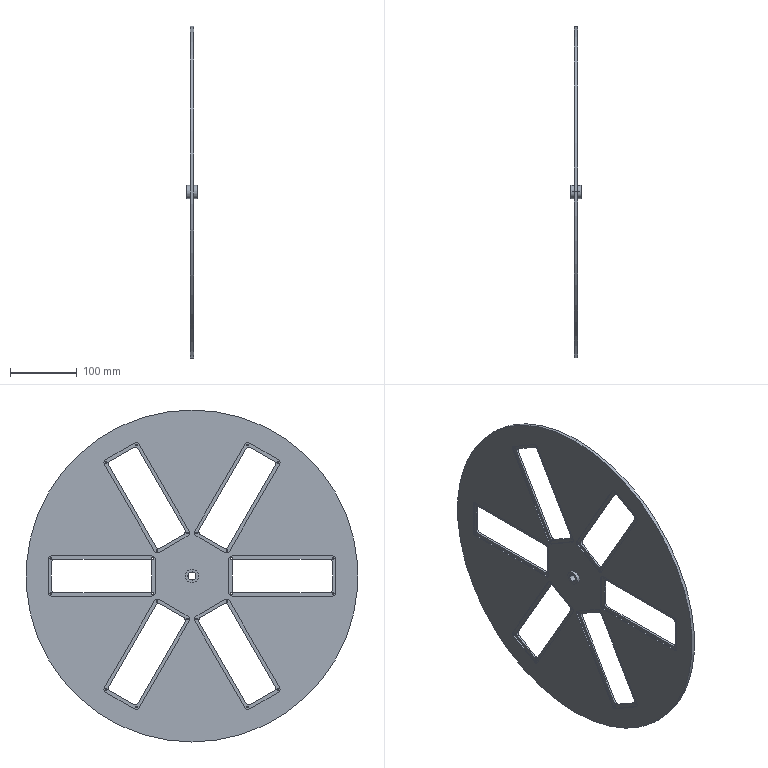Part | SolidWorks | features ICE 6, CirPattern 2, Fillet 2, Cut 1, Extrusion 1, HoleWzd 1 | 1 solid | 174 faces | box 15 x 496 x 496 mm | volume 717635 mm3 | cylinder 113 | plane 61 | commonest cylinder face diameters 10 x56 2.4 x48 20 x4 12 x3 496 x2